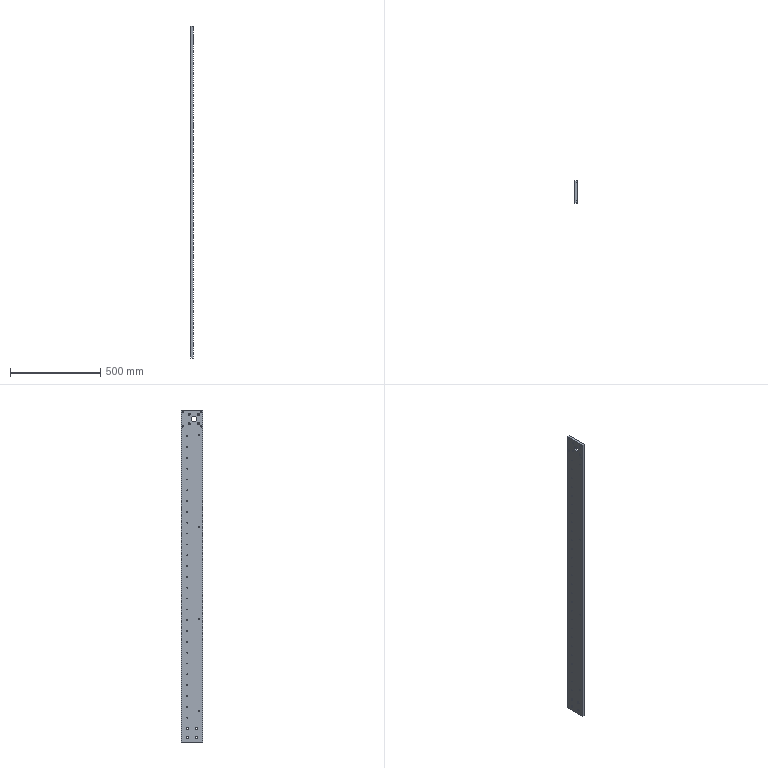Part | SolidWorks | features HoleWzd 5, ICE 2, LPattern 2, Extrusion 1 | 1 solid | 109 faces | box 14 x 120 x 1840 mm | volume 3046855 mm3 | cylinder 98 | plane 11 | commonest cylinder face diameters 4.2 x54 5 x8 6.6 x8 8.5 x8 11 x8 12.5 x8